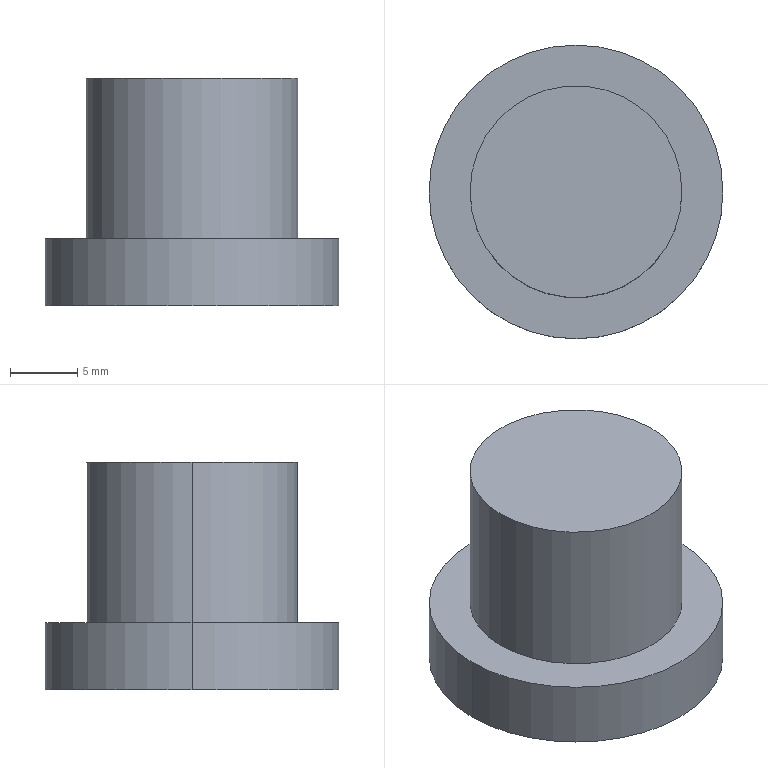Part | SolidWorks | features ICE 2, Extrusion 1 | 1 solid | 14 faces | box 21.9 x 21.9 x 17 mm | volume 3945 mm3 | plane 10 | cylinder 4 | commonest cylinder face diameters 15.8 x2 21.9 x2
STEP:
#1=CARTESIAN_POINT('',(-7.9,0.,17.));
#2=VERTEX_POINT('',#1);
#3=CARTESIAN_POINT('',(7.9,0.,17.));
#4=VERTEX_POINT('',#3);
#5=CARTESIAN_POINT('',(0.,0.,17.));
#6=DIRECTION('',(0.,0.,-1.));
#7=DIRECTION('',(-1.,0.,0.));
#8=AXIS2_PLACEMENT_3D('',#5,#6,#7);
#9=CIRCLE('',#8,7.9);
#10=EDGE_CURVE('',#2,#4,#9,.T.);
#11=ORIENTED_EDGE('',*,*,#10,.T.);
#12=CARTESIAN_POINT('',(7.9,0.,5.));
#13=VERTEX_POINT('',#12);
#14=CARTESIAN_POINT('',(7.9,0.,17.));
#15=DIRECTION('',(0.,0.,-1.));
#16=VECTOR('',#15,1000.);
#17=LINE('',#14,#16);
#18=EDGE_CURVE('',#4,#13,#17,.T.);
#19=ORIENTED_EDGE('',*,*,#18,.T.);
#20=CARTESIAN_POINT('',(-7.9,0.,5.));
#21=VERTEX_POINT('',#20);
#22=CARTESIAN_POINT('',(0.,0.,5.));
#23=DIRECTION('',(0.,0.,1.));
#24=DIRECTION('',(1.,0.,0.));
#25=AXIS2_PLACEMENT_3D('',#22,#23,#24);
#26=CIRCLE('',#25,7.9);
#27=EDGE_CURVE('',#13,#21,#26,.T.);
#28=ORIENTED_EDGE('',*,*,#27,.T.);
#29=CARTESIAN_POINT('',(-7.9,0.,17.));
#30=DIRECTION('',(0.,0.,-1.));
#31=VECTOR('',#30,1000.);
#32=LINE('',#29,#31);
#33=EDGE_CURVE('',#2,#21,#32,.T.);
#34=ORIENTED_EDGE('',*,*,#33,.F.);
#35=EDGE_LOOP('',(#11,#19,#28,#34));
#36=FACE_OUTER_BOUND('',#35,.T.);
#37=CARTESIAN_POINT('',(0.,0.,17.));
#38=DIRECTION('',(0.,0.,-1.));
#39=DIRECTION('',(-1.,0.,0.));
#40=AXIS2_PLACEMENT_3D('',#37,#38,#39);
#41=CYLINDRICAL_SURFACE('',#40,7.9);
#42=ADVANCED_FACE('',(#36),#41,.T.);
#43=CARTESIAN_POINT('',(10.95,0.,5.));
#44=VERTEX_POINT('',#43);
#45=CARTESIAN_POINT('',(-10.95,0.,5.));
#46=VERTEX_POINT('',#45);
#47=CARTESIAN_POINT('',(0.,0.,5.));
#48=DIRECTION('',(0.,0.,1.));
#49=DIRECTION('',(1.,0.,0.));
#50=AXIS2_PLACEMENT_3D('',#47,#48,#49);
#51=CIRCLE('',#50,10.95);
#52=EDGE_CURVE('',#44,#46,#51,.T.);
#53=ORIENTED_EDGE('',*,*,#52,.F.);
#54=CARTESIAN_POINT('',(10.95,0.,0.));
#55=VERTEX_POINT('',#54);
#56=CARTESIAN_POINT('',(10.95,0.,5.));
#57=DIRECTION('',(0.,0.,-1.));
#58=VECTOR('',#57,1000.);
#59=LINE('',#56,#58);
#60=EDGE_CURVE('',#44,#55,#59,.T.);
#61=ORIENTED_EDGE('',*,*,#60,.T.);
#62=CARTESIAN_POINT('',(-10.95,0.,0.));
#63=VERTEX_POINT('',#62);
#64=CARTESIAN_POINT('',(0.,0.,0.));
#65=DIRECTION('',(0.,0.,1.));
#66=DIRECTION('',(1.,0.,0.));
#67=AXIS2_PLACEMENT_3D('',#64,#65,#66);
#68=CIRCLE('',#67,10.95);
#69=EDGE_CURVE('',#55,#63,#68,.T.);
#70=ORIENTED_EDGE('',*,*,#69,.T.);
#71=CARTESIAN_POINT('',(-10.95,0.,5.));
#72=DIRECTION('',(0.,0.,-1.));
#73=VECTOR('',#72,1000.);
#74=LINE('',#71,#73);
#75=EDGE_CURVE('',#46,#63,#74,.T.);
#76=ORIENTED_EDGE('',*,*,#75,.F.);
#77=EDGE_LOOP('',(#53,#61,#70,#76));
#78=FACE_OUTER_BOUND('',#77,.T.);
#79=CARTESIAN_POINT('',(0.,0.,5.));
#80=DIRECTION('',(0.,0.,-1.));
#81=DIRECTION('',(-1.,0.,0.));
#82=AXIS2_PLACEMENT_3D('',#79,#80,#81);
#83=CYLINDRICAL_SURFACE('',#82,10.95);
#84=ADVANCED_FACE('',(#78),#83,.T.);
#85=ORIENTED_EDGE('',*,*,#60,.F.);
#86=CARTESIAN_POINT('',(0.,0.,5.));
#87=DIRECTION('',(0.,0.,1.));
#88=DIRECTION('',(1.,0.,0.));
#89=AXIS2_PLACEMENT_3D('',#86,#87,#88);
#90=CIRCLE('',#89,10.95);
#91=EDGE_CURVE('',#46,#44,#90,.T.);
#92=ORIENTED_EDGE('',*,*,#91,.F.);
#93=ORIENTED_EDGE('',*,*,#75,.T.);
#94=CARTESIAN_POINT('',(0.,0.,0.));
#95=DIRECTION('',(0.,0.,1.));
#96=DIRECTION('',(1.,0.,0.));
#97=AXIS2_PLACEMENT_3D('',#94,#95,#96);
#98=CIRCLE('',#97,10.95);
#99=EDGE_CURVE('',#63,#55,#98,.T.);
#100=ORIENTED_EDGE('',*,*,#99,.T.);
#101=EDGE_LOOP('',(#85,#92,#93,#100));
#102=FACE_OUTER_BOUND('',#101,.T.);
#103=CARTESIAN_POINT('',(0.,0.,5.));
#104=DIRECTION('',(0.,0.,-1.));
#105=DIRECTION('',(-1.,0.,0.));
#106=AXIS2_PLACEMENT_3D('',#103,#104,#105);
#107=CYLINDRICAL_SURFACE('',#106,10.95);
#108=ADVANCED_FACE('',(#102),#107,.T.);
#109=CARTESIAN_POINT('',(0.,0.,5.));
#110=DIRECTION('',(0.,0.,1.));
#111=DIRECTION('',(1.,0.,0.));
#112=AXIS2_PLACEMENT_3D('',#109,#110,#111);
#113=CIRCLE('',#112,7.9);
#114=EDGE_CURVE('',#21,#13,#113,.T.);
#115=ORIENTED_EDGE('',*,*,#114,.F.);
#116=ORIENTED_EDGE('',*,*,#27,.F.);
#117=EDGE_LOOP('',(#115,#116));
#118=FACE_BOUND('',#117,.T.);
#119=ORIENTED_EDGE('',*,*,#91,.T.);
#120=ORIENTED_EDGE('',*,*,#52,.T.);
#121=EDGE_LOOP('',(#119,#120));
#122=FACE_OUTER_BOUND('',#121,.T.);
#123=CARTESIAN_POINT('',(0.,0.,5.));
#124=DIRECTION('',(0.,0.,1.));
#125=DIRECTION('',(1.,0.,0.));
#126=AXIS2_PLACEMENT_3D('',#123,#124,#125);
#127=PLANE('',#126);
#128=ADVANCED_FACE('',(#118,#122),#127,.T.);
#129=CARTESIAN_POINT('',(0.,4.734,0.));
#130=VERTEX_POINT('',#129);
#131=CARTESIAN_POINT('',(4.1,2.367,0.));
#132=VERTEX_POINT('',#131);
#133=CARTESIAN_POINT('',(0.,4.734,0.));
#134=DIRECTION('',(0.866,-0.5,0.));
#135=VECTOR('',#134,1000.);
#136=LINE('',#133,#135);
#137=EDGE_CURVE('',#130,#132,#136,.T.);
#138=ORIENTED_EDGE('',*,*,#137,.F.);
#139=CARTESIAN_POINT('',(-4.1,2.367,0.));
#140=VERTEX_POINT('',#139);
#141=CARTESIAN_POINT('',(-4.1,2.367,0.));
#142=DIRECTION('',(0.866,0.5,0.));
#143=VECTOR('',#142,1000.);
#144=LINE('',#141,#143);
#145=EDGE_CURVE('',#140,#130,#144,.T.);
#146=ORIENTED_EDGE('',*,*,#145,.F.);
#147=CARTESIAN_POINT('',(-4.1,-2.367,0.));
#148=VERTEX_POINT('',#147);
#149=CARTESIAN_POINT('',(-4.1,-2.367,0.));
#150=DIRECTION('',(0.,1.,0.));
#151=VECTOR('',#150,1000.);
#152=LINE('',#149,#151);
#153=EDGE_CURVE('',#148,#140,#152,.T.);
#154=ORIENTED_EDGE('',*,*,#153,.F.);
#155=CARTESIAN_POINT('',(0.,-4.734,0.));
#156=VERTEX_POINT('',#155);
#157=CARTESIAN_POINT('',(0.,-4.734,0.));
#158=DIRECTION('',(-0.866,0.5,0.));
#159=VECTOR('',#158,1000.);
#160=LINE('',#157,#159);
#161=EDGE_CURVE('',#156,#148,#160,.T.);
#162=ORIENTED_EDGE('',*,*,#161,.F.);
#163=CARTESIAN_POINT('',(4.1,-2.367,0.));
#164=VERTEX_POINT('',#163);
#165=CARTESIAN_POINT('',(4.1,-2.367,0.));
#166=DIRECTION('',(-0.866,-0.5,0.));
#167=VECTOR('',#166,1000.);
#168=LINE('',#165,#167);
#169=EDGE_CURVE('',#164,#156,#168,.T.);
#170=ORIENTED_EDGE('',*,*,#169,.F.);
#171=CARTESIAN_POINT('',(4.1,2.367,0.));
#172=DIRECTION('',(0.,-1.,0.));
#173=VECTOR('',#172,1000.);
#174=LINE('',#171,#173);
#175=EDGE_CURVE('',#132,#164,#174,.T.);
#176=ORIENTED_EDGE('',*,*,#175,.F.);
#177=EDGE_LOOP('',(#138,#146,#154,#162,#170,#176));
#178=FACE_BOUND('',#177,.T.);
#179=ORIENTED_EDGE('',*,*,#99,.F.);
#180=ORIENTED_EDGE('',*,*,#69,.F.);
#181=EDGE_LOOP('',(#179,#180));
#182=FACE_OUTER_BOUND('',#181,.T.);
#183=CARTESIAN_POINT('',(0.,0.,0.));
#184=DIRECTION('',(0.,0.,1.));
#185=DIRECTION('',(1.,0.,0.));
#186=AXIS2_PLACEMENT_3D('',#183,#184,#185);
#187=PLANE('',#186);
#188=ADVANCED_FACE('',(#178,#182),#187,.F.);
#189=ORIENTED_EDGE('',*,*,#18,.F.);
#190=CARTESIAN_POINT('',(0.,0.,17.));
#191=DIRECTION('',(0.,0.,-1.));
#192=DIRECTION('',(-1.,0.,0.));
#193=AXIS2_PLACEMENT_3D('',#190,#191,#192);
#194=CIRCLE('',#193,7.9);
#195=EDGE_CURVE('',#4,#2,#194,.T.);
#196=ORIENTED_EDGE('',*,*,#195,.T.);
#197=ORIENTED_EDGE('',*,*,#33,.T.);
#198=ORIENTED_EDGE('',*,*,#114,.T.);
#199=EDGE_LOOP('',(#189,#196,#197,#198));
#200=FACE_OUTER_BOUND('',#199,.T.);
#201=CARTESIAN_POINT('',(0.,0.,17.));
#202=DIRECTION('',(0.,0.,-1.));
#203=DIRECTION('',(-1.,0.,0.));
#204=AXIS2_PLACEMENT_3D('',#201,#202,#203);
#205=CYLINDRICAL_SURFACE('',#204,7.9);
#206=ADVANCED_FACE('',(#200),#205,.T.);
#207=ORIENTED_EDGE('',*,*,#10,.F.);
#208=ORIENTED_EDGE('',*,*,#195,.F.);
#209=EDGE_LOOP('',(#207,#208));
#210=FACE_OUTER_BOUND('',#209,.T.);
#211=CARTESIAN_POINT('',(0.,0.,17.));
#212=DIRECTION('',(0.,0.,-1.));
#213=DIRECTION('',(-1.,0.,0.));
#214=AXIS2_PLACEMENT_3D('',#211,#212,#213);
#215=PLANE('',#214);
#216=ADVANCED_FACE('',(#210),#215,.F.);
#217=ORIENTED_EDGE('',*,*,#145,.T.);
#218=CARTESIAN_POINT('',(0.,4.734,5.));
#219=VERTEX_POINT('',#218);
#220=CARTESIAN_POINT('',(0.,4.734,5.));
#221=DIRECTION('',(0.,0.,-1.));
#222=VECTOR('',#221,1000.);
#223=LINE('',#220,#222);
#224=EDGE_CURVE('',#219,#130,#223,.T.);
#225=ORIENTED_EDGE('',*,*,#224,.F.);
#226=CARTESIAN_POINT('',(-4.1,2.367,5.));
#227=VERTEX_POINT('',#226);
#228=CARTESIAN_POINT('',(-4.1,2.367,5.));
#229=DIRECTION('',(0.866,0.5,0.));
#230=VECTOR('',#229,1000.);
#231=LINE('',#228,#230);
#232=EDGE_CURVE('',#227,#219,#231,.T.);
#233=ORIENTED_EDGE('',*,*,#232,.F.);
#234=CARTESIAN_POINT('',(-4.1,2.367,5.));
#235=DIRECTION('',(0.,0.,-1.));
#236=VECTOR('',#235,1000.);
#237=LINE('',#234,#236);
#238=EDGE_CURVE('',#227,#140,#237,.T.);
#239=ORIENTED_EDGE('',*,*,#238,.T.);
#240=EDGE_LOOP('',(#217,#225,#233,#239));
#241=FACE_OUTER_BOUND('',#240,.T.);
#242=CARTESIAN_POINT('',(-4.1,2.367,5.));
#243=DIRECTION('',(-0.5,0.866,0.));
#244=DIRECTION('',(-0.866,-0.5,0.));
#245=AXIS2_PLACEMENT_3D('',#242,#243,#244);
#246=PLANE('',#245);
#247=ADVANCED_FACE('',(#241),#246,.F.);
#248=ORIENTED_EDGE('',*,*,#153,.T.);
#249=ORIENTED_EDGE('',*,*,#238,.F.);
#250=CARTESIAN_POINT('',(-4.1,-2.367,5.));
#251=VERTEX_POINT('',#250);
#252=CARTESIAN_POINT('',(-4.1,-2.367,5.));
#253=DIRECTION('',(0.,1.,0.));
#254=VECTOR('',#253,1000.);
#255=LINE('',#252,#254);
#256=EDGE_CURVE('',#251,#227,#255,.T.);
#257=ORIENTED_EDGE('',*,*,#256,.F.);
#258=CARTESIAN_POINT('',(-4.1,-2.367,5.));
#259=DIRECTION('',(0.,0.,-1.));
#260=VECTOR('',#259,1000.);
#261=LINE('',#258,#260);
#262=EDGE_CURVE('',#251,#148,#261,.T.);
#263=ORIENTED_EDGE('',*,*,#262,.T.);
#264=EDGE_LOOP('',(#248,#249,#257,#263));
#265=FACE_OUTER_BOUND('',#264,.T.);
#266=CARTESIAN_POINT('',(-4.1,-2.367,5.));
#267=DIRECTION('',(-1.,0.,0.));
#268=DIRECTION('',(0.,-1.,0.));
#269=AXIS2_PLACEMENT_3D('',#266,#267,#268);
#270=PLANE('',#269);
#271=ADVANCED_FACE('',(#265),#270,.F.);
#272=ORIENTED_EDGE('',*,*,#161,.T.);
#273=ORIENTED_EDGE('',*,*,#262,.F.);
#274=CARTESIAN_POINT('',(0.,-4.734,5.));
#275=VERTEX_POINT('',#274);
#276=CARTESIAN_POINT('',(0.,-4.734,5.));
#277=DIRECTION('',(-0.866,0.5,0.));
#278=VECTOR('',#277,1000.);
#279=LINE('',#276,#278);
#280=EDGE_CURVE('',#275,#251,#279,.T.);
#281=ORIENTED_EDGE('',*,*,#280,.F.);
#282=CARTESIAN_POINT('',(0.,-4.734,5.));
#283=DIRECTION('',(0.,0.,-1.));
#284=VECTOR('',#283,1000.);
#285=LINE('',#282,#284);
#286=EDGE_CURVE('',#275,#156,#285,.T.);
#287=ORIENTED_EDGE('',*,*,#286,.T.);
#288=EDGE_LOOP('',(#272,#273,#281,#287));
#289=FACE_OUTER_BOUND('',#288,.T.);
#290=CARTESIAN_POINT('',(0.,-4.734,5.));
#291=DIRECTION('',(-0.5,-0.866,0.));
#292=DIRECTION('',(0.866,-0.5,0.));
#293=AXIS2_PLACEMENT_3D('',#290,#291,#292);
#294=PLANE('',#293);
#295=ADVANCED_FACE('',(#289),#294,.F.);
#296=ORIENTED_EDGE('',*,*,#169,.T.);
#297=ORIENTED_EDGE('',*,*,#286,.F.);
#298=CARTESIAN_POINT('',(4.1,-2.367,5.));
#299=VERTEX_POINT('',#298);
#300=CARTESIAN_POINT('',(4.1,-2.367,5.));
#301=DIRECTION('',(-0.866,-0.5,0.));
#302=VECTOR('',#301,1000.);
#303=LINE('',#300,#302);
#304=EDGE_CURVE('',#299,#275,#303,.T.);
#305=ORIENTED_EDGE('',*,*,#304,.F.);
#306=CARTESIAN_POINT('',(4.1,-2.367,5.));
#307=DIRECTION('',(0.,0.,-1.));
#308=VECTOR('',#307,1000.);
#309=LINE('',#306,#308);
#310=EDGE_CURVE('',#299,#164,#309,.T.);
#311=ORIENTED_EDGE('',*,*,#310,.T.);
#312=EDGE_LOOP('',(#296,#297,#305,#311));
#313=FACE_OUTER_BOUND('',#312,.T.);
#314=CARTESIAN_POINT('',(4.1,-2.367,5.));
#315=DIRECTION('',(0.5,-0.866,0.));
#316=DIRECTION('',(0.866,0.5,0.));
#317=AXIS2_PLACEMENT_3D('',#314,#315,#316);
#318=PLANE('',#317);
#319=ADVANCED_FACE('',(#313),#318,.F.);
#320=ORIENTED_EDGE('',*,*,#175,.T.);
#321=ORIENTED_EDGE('',*,*,#310,.F.);
#322=CARTESIAN_POINT('',(4.1,2.367,5.));
#323=VERTEX_POINT('',#322);
#324=CARTESIAN_POINT('',(4.1,2.367,5.));
#325=DIRECTION('',(0.,-1.,0.));
#326=VECTOR('',#325,1000.);
#327=LINE('',#324,#326);
#328=EDGE_CURVE('',#323,#299,#327,.T.);
#329=ORIENTED_EDGE('',*,*,#328,.F.);
#330=CARTESIAN_POINT('',(4.1,2.367,5.));
#331=DIRECTION('',(0.,0.,-1.));
#332=VECTOR('',#331,1000.);
#333=LINE('',#330,#332);
#334=EDGE_CURVE('',#323,#132,#333,.T.);
#335=ORIENTED_EDGE('',*,*,#334,.T.);
#336=EDGE_LOOP('',(#320,#321,#329,#335));
#337=FACE_OUTER_BOUND('',#336,.T.);
#338=CARTESIAN_POINT('',(4.1,2.367,5.));
#339=DIRECTION('',(1.,0.,0.));
#340=DIRECTION('',(0.,1.,0.));
#341=AXIS2_PLACEMENT_3D('',#338,#339,#340);
#342=PLANE('',#341);
#343=ADVANCED_FACE('',(#337),#342,.F.);
#344=ORIENTED_EDGE('',*,*,#137,.T.);
#345=ORIENTED_EDGE('',*,*,#334,.F.);
#346=CARTESIAN_POINT('',(0.,4.734,5.));
#347=DIRECTION('',(0.866,-0.5,0.));
#348=VECTOR('',#347,1000.);
#349=LINE('',#346,#348);
#350=EDGE_CURVE('',#219,#323,#349,.T.);
#351=ORIENTED_EDGE('',*,*,#350,.F.);
#352=ORIENTED_EDGE('',*,*,#224,.T.);
#353=EDGE_LOOP('',(#344,#345,#351,#352));
#354=FACE_OUTER_BOUND('',#353,.T.);
#355=CARTESIAN_POINT('',(0.,4.734,5.));
#356=DIRECTION('',(0.5,0.866,0.));
#357=DIRECTION('',(-0.866,0.5,0.));
#358=AXIS2_PLACEMENT_3D('',#355,#356,#357);
#359=PLANE('',#358);
#360=ADVANCED_FACE('',(#354),#359,.F.);
#361=ORIENTED_EDGE('',*,*,#232,.T.);
#362=ORIENTED_EDGE('',*,*,#350,.T.);
#363=ORIENTED_EDGE('',*,*,#328,.T.);
#364=ORIENTED_EDGE('',*,*,#304,.T.);
#365=ORIENTED_EDGE('',*,*,#280,.T.);
#366=ORIENTED_EDGE('',*,*,#256,.T.);
#367=EDGE_LOOP('',(#361,#362,#363,#364,#365,#366));
#368=FACE_OUTER_BOUND('',#367,.T.);
#369=CARTESIAN_POINT('',(0.,0.,5.));
#370=DIRECTION('',(0.,0.,-1.));
#371=DIRECTION('',(-1.,0.,0.));
#372=AXIS2_PLACEMENT_3D('',#369,#370,#371);
#373=PLANE('',#372);
#374=ADVANCED_FACE('',(#368),#373,.T.);
#375=CLOSED_SHELL('',(#42,#84,#108,#128,#188,#206,#216,#247,#271,#295,#319,#343,#360,#374));
#376=MANIFOLD_SOLID_BREP('',#375);
#377=CARTESIAN_POINT('',(0.,0.,0.));
#378=DIRECTION('',(0.,0.,1.));
#379=DIRECTION('',(1.,0.,0.));
#380=AXIS2_PLACEMENT_3D('',#377,#378,#379);
#381=(LENGTH_UNIT()NAMED_UNIT(*)SI_UNIT(.MILLI.,.METRE.));
#382=UNCERTAINTY_MEASURE_WITH_UNIT(LENGTH_MEASURE(0.00001),#381,'','');
#383=(NAMED_UNIT(*)PLANE_ANGLE_UNIT()SI_UNIT($,.RADIAN.));
#384=(NAMED_UNIT(*)SI_UNIT($,.STERADIAN.)SOLID_ANGLE_UNIT());
#385=(GEOMETRIC_REPRESENTATION_CONTEXT(3)GLOBAL_UNCERTAINTY_ASSIGNED_CONTEXT((#382))GLOBAL_UNIT_ASSIGNED_CONTEXT((#381,#383,#384))REPRESENTATION_CONTEXT('',''));
#386=ADVANCED_BREP_SHAPE_REPRESENTATION('',(#376,#380),#385);